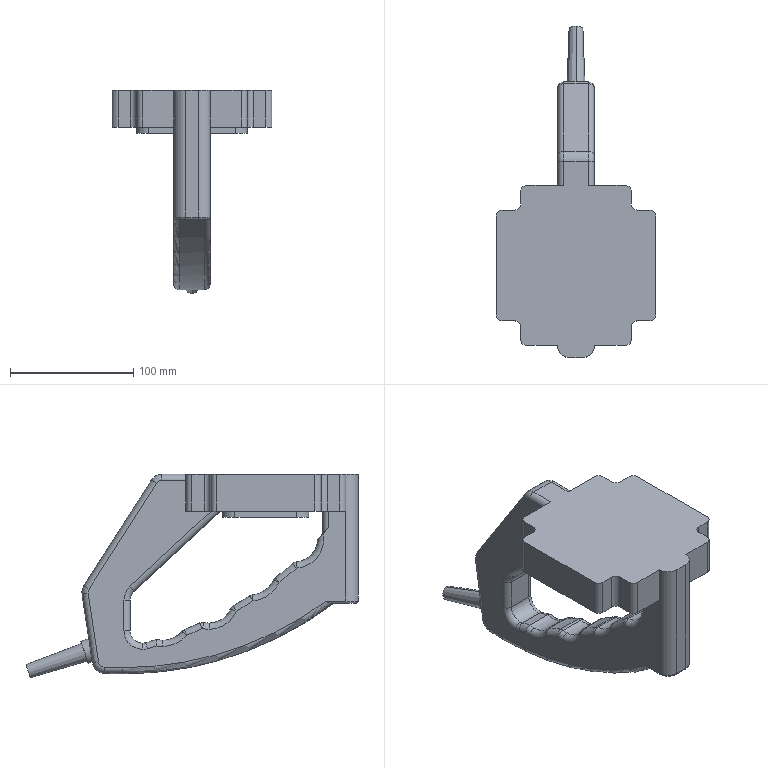Part | SolidWorks | features Fillet 14, ICE 12, CirPattern 2, Extrusion 1, MirrorPattern 1, RefAxis 1, Revolution 1 | 1 solid | 137 faces | box 130 x 269.835 x 165.306 mm | volume 953588 mm3 | cylinder 56 | torus 34 | plane 31 | sphere 12 | cone 4 | commonest cylinder face diameters 10 x30 20 x11 620.762 x5 4 x3 18.846 x2 36.81 x1